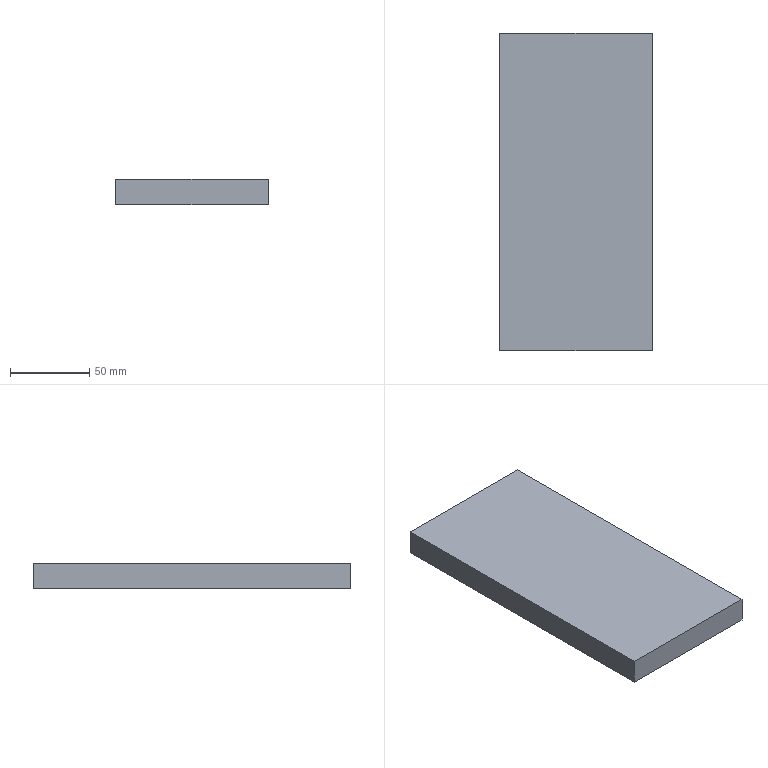Part | SolidWorks | features Extrusion 1 | 1 solid | 6 faces | box 96 x 200 x 16 mm | volume 307200 mm3 | plane 6
STEP:
#1=CARTESIAN_POINT('',(48.,-100.,-8.));
#2=VERTEX_POINT('',#1);
#3=CARTESIAN_POINT('',(48.,100.,-8.));
#4=VERTEX_POINT('',#3);
#5=CARTESIAN_POINT('',(48.,-100.,-8.));
#6=DIRECTION('',(0.,1.,0.));
#7=VECTOR('',#6,1000.);
#8=LINE('',#5,#7);
#9=EDGE_CURVE('',#2,#4,#8,.T.);
#10=ORIENTED_EDGE('',*,*,#9,.T.);
#11=CARTESIAN_POINT('',(48.,100.,8.));
#12=VERTEX_POINT('',#11);
#13=CARTESIAN_POINT('',(48.,100.,8.));
#14=DIRECTION('',(0.,0.,-1.));
#15=VECTOR('',#14,1000.);
#16=LINE('',#13,#15);
#17=EDGE_CURVE('',#12,#4,#16,.T.);
#18=ORIENTED_EDGE('',*,*,#17,.F.);
#19=CARTESIAN_POINT('',(48.,-100.,8.));
#20=VERTEX_POINT('',#19);
#21=CARTESIAN_POINT('',(48.,-100.,8.));
#22=DIRECTION('',(0.,1.,0.));
#23=VECTOR('',#22,1000.);
#24=LINE('',#21,#23);
#25=EDGE_CURVE('',#20,#12,#24,.T.);
#26=ORIENTED_EDGE('',*,*,#25,.F.);
#27=CARTESIAN_POINT('',(48.,-100.,8.));
#28=DIRECTION('',(0.,0.,-1.));
#29=VECTOR('',#28,1000.);
#30=LINE('',#27,#29);
#31=EDGE_CURVE('',#20,#2,#30,.T.);
#32=ORIENTED_EDGE('',*,*,#31,.T.);
#33=EDGE_LOOP('',(#10,#18,#26,#32));
#34=FACE_OUTER_BOUND('',#33,.T.);
#35=CARTESIAN_POINT('',(48.,-100.,8.));
#36=DIRECTION('',(-1.,0.,0.));
#37=DIRECTION('',(0.,-1.,0.));
#38=AXIS2_PLACEMENT_3D('',#35,#36,#37);
#39=PLANE('',#38);
#40=ADVANCED_FACE('',(#34),#39,.F.);
#41=CARTESIAN_POINT('',(-48.,100.,-8.));
#42=VERTEX_POINT('',#41);
#43=CARTESIAN_POINT('',(48.,100.,-8.));
#44=DIRECTION('',(-1.,0.,0.));
#45=VECTOR('',#44,1000.);
#46=LINE('',#43,#45);
#47=EDGE_CURVE('',#4,#42,#46,.T.);
#48=ORIENTED_EDGE('',*,*,#47,.T.);
#49=CARTESIAN_POINT('',(-48.,100.,8.));
#50=VERTEX_POINT('',#49);
#51=CARTESIAN_POINT('',(-48.,100.,8.));
#52=DIRECTION('',(0.,0.,-1.));
#53=VECTOR('',#52,1000.);
#54=LINE('',#51,#53);
#55=EDGE_CURVE('',#50,#42,#54,.T.);
#56=ORIENTED_EDGE('',*,*,#55,.F.);
#57=CARTESIAN_POINT('',(48.,100.,8.));
#58=DIRECTION('',(-1.,0.,0.));
#59=VECTOR('',#58,1000.);
#60=LINE('',#57,#59);
#61=EDGE_CURVE('',#12,#50,#60,.T.);
#62=ORIENTED_EDGE('',*,*,#61,.F.);
#63=ORIENTED_EDGE('',*,*,#17,.T.);
#64=EDGE_LOOP('',(#48,#56,#62,#63));
#65=FACE_OUTER_BOUND('',#64,.T.);
#66=CARTESIAN_POINT('',(48.,100.,8.));
#67=DIRECTION('',(0.,-1.,0.));
#68=DIRECTION('',(1.,0.,0.));
#69=AXIS2_PLACEMENT_3D('',#66,#67,#68);
#70=PLANE('',#69);
#71=ADVANCED_FACE('',(#65),#70,.F.);
#72=CARTESIAN_POINT('',(-48.,-100.,-8.));
#73=VERTEX_POINT('',#72);
#74=CARTESIAN_POINT('',(-48.,100.,-8.));
#75=DIRECTION('',(0.,-1.,0.));
#76=VECTOR('',#75,1000.);
#77=LINE('',#74,#76);
#78=EDGE_CURVE('',#42,#73,#77,.T.);
#79=ORIENTED_EDGE('',*,*,#78,.T.);
#80=CARTESIAN_POINT('',(-48.,-100.,8.));
#81=VERTEX_POINT('',#80);
#82=CARTESIAN_POINT('',(-48.,-100.,8.));
#83=DIRECTION('',(0.,0.,-1.));
#84=VECTOR('',#83,1000.);
#85=LINE('',#82,#84);
#86=EDGE_CURVE('',#81,#73,#85,.T.);
#87=ORIENTED_EDGE('',*,*,#86,.F.);
#88=CARTESIAN_POINT('',(-48.,100.,8.));
#89=DIRECTION('',(0.,-1.,0.));
#90=VECTOR('',#89,1000.);
#91=LINE('',#88,#90);
#92=EDGE_CURVE('',#50,#81,#91,.T.);
#93=ORIENTED_EDGE('',*,*,#92,.F.);
#94=ORIENTED_EDGE('',*,*,#55,.T.);
#95=EDGE_LOOP('',(#79,#87,#93,#94));
#96=FACE_OUTER_BOUND('',#95,.T.);
#97=CARTESIAN_POINT('',(-48.,100.,8.));
#98=DIRECTION('',(1.,0.,0.));
#99=DIRECTION('',(0.,1.,0.));
#100=AXIS2_PLACEMENT_3D('',#97,#98,#99);
#101=PLANE('',#100);
#102=ADVANCED_FACE('',(#96),#101,.F.);
#103=CARTESIAN_POINT('',(-48.,-100.,-8.));
#104=DIRECTION('',(1.,0.,0.));
#105=VECTOR('',#104,1000.);
#106=LINE('',#103,#105);
#107=EDGE_CURVE('',#73,#2,#106,.T.);
#108=ORIENTED_EDGE('',*,*,#107,.T.);
#109=ORIENTED_EDGE('',*,*,#31,.F.);
#110=CARTESIAN_POINT('',(-48.,-100.,8.));
#111=DIRECTION('',(1.,0.,0.));
#112=VECTOR('',#111,1000.);
#113=LINE('',#110,#112);
#114=EDGE_CURVE('',#81,#20,#113,.T.);
#115=ORIENTED_EDGE('',*,*,#114,.F.);
#116=ORIENTED_EDGE('',*,*,#86,.T.);
#117=EDGE_LOOP('',(#108,#109,#115,#116));
#118=FACE_OUTER_BOUND('',#117,.T.);
#119=CARTESIAN_POINT('',(-48.,-100.,8.));
#120=DIRECTION('',(0.,1.,0.));
#121=DIRECTION('',(0.,0.,1.));
#122=AXIS2_PLACEMENT_3D('',#119,#120,#121);
#123=PLANE('',#122);
#124=ADVANCED_FACE('',(#118),#123,.F.);
#125=ORIENTED_EDGE('',*,*,#25,.T.);
#126=ORIENTED_EDGE('',*,*,#61,.T.);
#127=ORIENTED_EDGE('',*,*,#92,.T.);
#128=ORIENTED_EDGE('',*,*,#114,.T.);
#129=EDGE_LOOP('',(#125,#126,#127,#128));
#130=FACE_OUTER_BOUND('',#129,.T.);
#131=CARTESIAN_POINT('',(48.,100.,8.));
#132=DIRECTION('',(0.,0.,1.));
#133=DIRECTION('',(1.,0.,0.));
#134=AXIS2_PLACEMENT_3D('',#131,#132,#133);
#135=PLANE('',#134);
#136=ADVANCED_FACE('',(#130),#135,.T.);
#137=ORIENTED_EDGE('',*,*,#9,.F.);
#138=ORIENTED_EDGE('',*,*,#107,.F.);
#139=ORIENTED_EDGE('',*,*,#78,.F.);
#140=ORIENTED_EDGE('',*,*,#47,.F.);
#141=EDGE_LOOP('',(#137,#138,#139,#140));
#142=FACE_OUTER_BOUND('',#141,.T.);
#143=CARTESIAN_POINT('',(48.,100.,-8.));
#144=DIRECTION('',(0.,0.,1.));
#145=DIRECTION('',(1.,0.,0.));
#146=AXIS2_PLACEMENT_3D('',#143,#144,#145);
#147=PLANE('',#146);
#148=ADVANCED_FACE('',(#142),#147,.F.);
#149=CLOSED_SHELL('',(#40,#71,#102,#124,#136,#148));
#150=MANIFOLD_SOLID_BREP('',#149);
#151=CARTESIAN_POINT('',(0.,0.,0.));
#152=DIRECTION('',(0.,0.,1.));
#153=DIRECTION('',(1.,0.,0.));
#154=AXIS2_PLACEMENT_3D('',#151,#152,#153);
#155=(LENGTH_UNIT()NAMED_UNIT(*)SI_UNIT(.MILLI.,.METRE.));
#156=UNCERTAINTY_MEASURE_WITH_UNIT(LENGTH_MEASURE(0.00001),#155,'','');
#157=(NAMED_UNIT(*)PLANE_ANGLE_UNIT()SI_UNIT($,.RADIAN.));
#158=(NAMED_UNIT(*)SI_UNIT($,.STERADIAN.)SOLID_ANGLE_UNIT());
#159=(GEOMETRIC_REPRESENTATION_CONTEXT(3)GLOBAL_UNCERTAINTY_ASSIGNED_CONTEXT((#156))GLOBAL_UNIT_ASSIGNED_CONTEXT((#155,#157,#158))REPRESENTATION_CONTEXT('',''));
#160=ADVANCED_BREP_SHAPE_REPRESENTATION('',(#150,#154),#159);